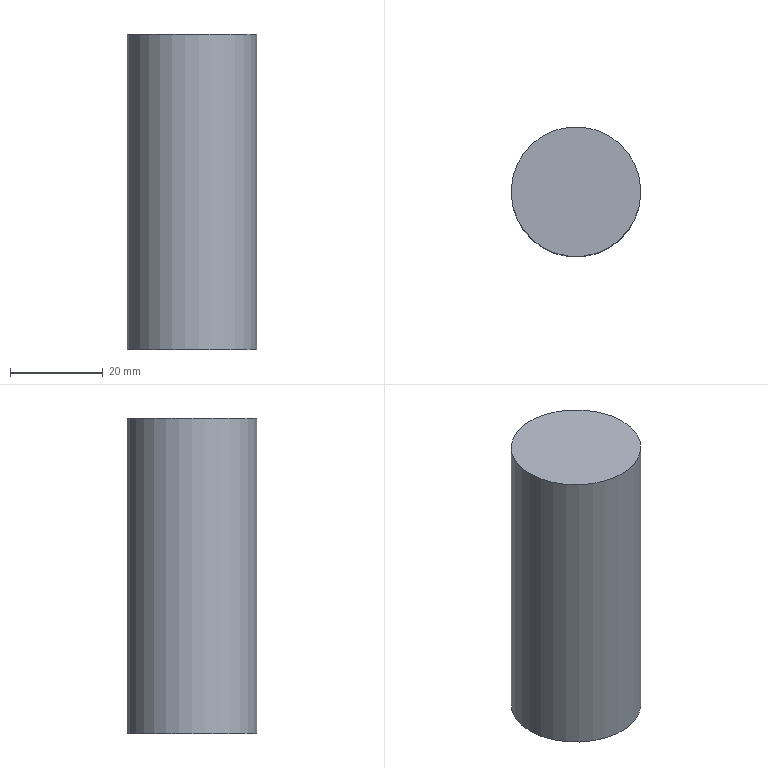Part | NX | features solid 2 | 1 solid | 3 faces | box 28 x 28 x 68 mm | volume 41871 mm3 | plane 2 | cylinder 1 | commonest cylinder face diameters 28 x1
STEP:
#1=CARTESIAN_POINT('',(-76.,255.,142.));
#2=VERTEX_POINT('',#1);
#3=CARTESIAN_POINT('',(-90.,255.,142.));
#4=DIRECTION('',(0.,0.,1.));
#5=DIRECTION('',(1.,0.,0.));
#6=AXIS2_PLACEMENT_3D('',#3,#4,#5);
#7=CIRCLE('',#6,14.);
#8=EDGE_CURVE('',#2,#2,#7,.T.);
#9=ORIENTED_EDGE('',*,*,#8,.T.);
#10=EDGE_LOOP('',(#9));
#11=FACE_BOUND('',#10,.T.);
#12=CARTESIAN_POINT('',(-104.,255.,210.));
#13=VERTEX_POINT('',#12);
#14=CARTESIAN_POINT('',(-90.,255.,210.));
#15=DIRECTION('',(0.,0.,-1.));
#16=DIRECTION('',(-1.,0.,0.));
#17=AXIS2_PLACEMENT_3D('',#14,#15,#16);
#18=CIRCLE('',#17,14.);
#19=EDGE_CURVE('',#13,#13,#18,.F.);
#20=ORIENTED_EDGE('',*,*,#19,.F.);
#21=EDGE_LOOP('',(#20));
#22=FACE_BOUND('',#21,.T.);
#23=CARTESIAN_POINT('',(-90.,255.,210.76));
#24=DIRECTION('',(0.,0.,-1.));
#25=DIRECTION('',(0.,1.,0.));
#26=AXIS2_PLACEMENT_3D('',#23,#24,#25);
#27=CYLINDRICAL_SURFACE('',#26,14.);
#28=ADVANCED_FACE('',(#11,#22),#27,.T.);
#29=ORIENTED_EDGE('',*,*,#19,.T.);
#30=EDGE_LOOP('',(#29));
#31=FACE_BOUND('',#30,.T.);
#32=CARTESIAN_POINT('',(-90.,259.348,210.));
#33=DIRECTION('',(0.,0.,-1.));
#34=DIRECTION('',(0.,1.,0.));
#35=AXIS2_PLACEMENT_3D('',#32,#33,#34);
#36=PLANE('',#35);
#37=ADVANCED_FACE('',(#31),#36,.F.);
#38=ORIENTED_EDGE('',*,*,#8,.F.);
#39=EDGE_LOOP('',(#38));
#40=FACE_BOUND('',#39,.T.);
#41=CARTESIAN_POINT('',(-90.,259.348,142.));
#42=DIRECTION('',(0.,0.,-1.));
#43=DIRECTION('',(0.,1.,0.));
#44=AXIS2_PLACEMENT_3D('',#41,#42,#43);
#45=PLANE('',#44);
#46=ADVANCED_FACE('',(#40),#45,.T.);
#47=CLOSED_SHELL('',(#28,#37,#46));
#48=MANIFOLD_SOLID_BREP('',#47);
#49=(LENGTH_UNIT()NAMED_UNIT(*)SI_UNIT(.MILLI.,.METRE.));
#50=UNCERTAINTY_MEASURE_WITH_UNIT(LENGTH_MEASURE(0.00001),#49,'','');
#51=(NAMED_UNIT(*)PLANE_ANGLE_UNIT()SI_UNIT($,.RADIAN.));
#52=(NAMED_UNIT(*)SI_UNIT($,.STERADIAN.)SOLID_ANGLE_UNIT());
#53=(GEOMETRIC_REPRESENTATION_CONTEXT(3)GLOBAL_UNCERTAINTY_ASSIGNED_CONTEXT((#50))GLOBAL_UNIT_ASSIGNED_CONTEXT((#49,#51,#52))REPRESENTATION_CONTEXT('',''));
#54=ADVANCED_BREP_SHAPE_REPRESENTATION('',(#48),#53);